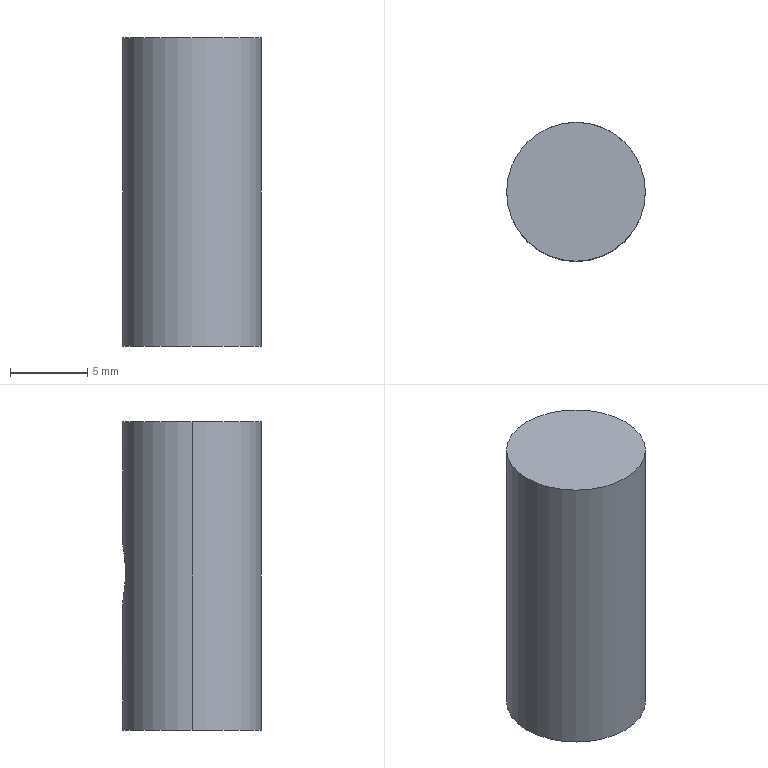Part | SolidWorks | features 3DProfileFeature 1, Extrusion 1, HoleWzd 1 | 1 solid | 8 faces | box 9 x 9 x 20 mm | volume 1148 mm3 | cylinder 4 | cone 2 | plane 2 | commonest cylinder face diameters 5 x2 9 x2
STEP:
#1=CARTESIAN_POINT('',(-0.8907,-2.867,10.19));
#2=VERTEX_POINT('',#1);
#3=CARTESIAN_POINT('',(-2.832,-0.6908,10.19));
#4=VERTEX_POINT('',#3);
#5=CARTESIAN_POINT('',(-2.832,-0.6908,10.19));
#6=DIRECTION('',(-0.6658,0.7462,0.));
#7=VECTOR('',#6,1000.);
#8=LINE('',#5,#7);
#9=EDGE_CURVE('',#2,#4,#8,.T.);
#10=ORIENTED_EDGE('',*,*,#9,.F.);
#11=CARTESIAN_POINT('',(1.942,-2.174,10.19));
#12=VERTEX_POINT('',#11);
#13=CARTESIAN_POINT('',(1.942,-2.174,10.19));
#14=DIRECTION('',(0.9714,0.2375,0.));
#15=VECTOR('',#14,1000.);
#16=LINE('',#13,#15);
#17=EDGE_CURVE('',#2,#12,#16,.T.);
#18=ORIENTED_EDGE('',*,*,#17,.T.);
#19=CARTESIAN_POINT('',(-0.445,-1.432,10.19));
#20=DIRECTION('',(0.2967,0.955,0.));
#21=DIRECTION('',(-0.955,0.2967,0.));
#22=AXIS2_PLACEMENT_3D('',#19,#20,#21);
#23=CIRCLE('',#22,2.5);
#24=EDGE_CURVE('',#12,#4,#23,.T.);
#25=ORIENTED_EDGE('',*,*,#24,.T.);
#26=EDGE_LOOP('',(#10,#18,#25));
#27=FACE_OUTER_BOUND('',#26,.T.);
#28=CARTESIAN_POINT('',(-0.445,-1.432,10.19));
#29=DIRECTION('',(0.2967,0.955,0.));
#30=DIRECTION('',(-0.955,0.2967,0.));
#31=AXIS2_PLACEMENT_3D('',#28,#29,#30);
#32=CONICAL_SURFACE('',#31,2.5,1.03);
#33=ADVANCED_FACE('',(#27),#32,.F.);
#34=ORIENTED_EDGE('',*,*,#24,.F.);
#35=CARTESIAN_POINT('',(3.498,2.831,10.19));
#36=VERTEX_POINT('',#35);
#37=CARTESIAN_POINT('',(3.723,3.556,10.19));
#38=DIRECTION('',(0.2967,0.955,0.));
#39=VECTOR('',#38,1000.);
#40=LINE('',#37,#39);
#41=EDGE_CURVE('',#12,#36,#40,.T.);
#42=ORIENTED_EDGE('',*,*,#41,.T.);
#43=CARTESIAN_POINT('',(-1.277,4.315,10.19));
#44=VERTEX_POINT('',#43);
#45=CARTESIAN_POINT('',(-1.277,4.315,10.19));
#46=CARTESIAN_POINT('',(-1.277,4.315,10.021));
#47=CARTESIAN_POINT('',(-1.258,4.321,9.855));
#48=CARTESIAN_POINT('',(-1.182,4.342,9.531));
#49=CARTESIAN_POINT('',(-1.126,4.358,9.371));
#50=CARTESIAN_POINT('',(-0.9113,4.409,8.921));
#51=CARTESIAN_POINT('',(-0.7062,4.451,8.649));
#52=CARTESIAN_POINT('',(-0.3401,4.489,8.31));
#53=CARTESIAN_POINT('',(-0.2061,4.497,8.207));
#54=CARTESIAN_POINT('',(0.07581,4.502,8.026));
#55=CARTESIAN_POINT('',(0.223,4.497,7.949));
#56=CARTESIAN_POINT('',(0.5298,4.471,7.823));
#57=CARTESIAN_POINT('',(0.6916,4.45,7.773));
#58=CARTESIAN_POINT('',(1.013,4.388,7.707));
#59=CARTESIAN_POINT('',(1.173,4.348,7.69));
#60=CARTESIAN_POINT('',(1.493,4.248,7.69));
#61=CARTESIAN_POINT('',(1.652,4.189,7.707));
#62=CARTESIAN_POINT('',(1.951,4.058,7.773));
#63=CARTESIAN_POINT('',(2.096,3.985,7.822));
#64=CARTESIAN_POINT('',(2.366,3.831,7.95));
#65=CARTESIAN_POINT('',(2.49,3.751,8.027));
#66=CARTESIAN_POINT('',(2.721,3.587,8.209));
#67=CARTESIAN_POINT('',(2.826,3.504,8.313));
#68=CARTESIAN_POINT('',(3.106,3.266,8.652));
#69=CARTESIAN_POINT('',(3.251,3.115,8.924));
#70=CARTESIAN_POINT('',(3.397,2.952,9.373));
#71=CARTESIAN_POINT('',(3.435,2.907,9.532));
#72=CARTESIAN_POINT('',(3.485,2.847,9.858));
#73=CARTESIAN_POINT('',(3.498,2.831,10.023));
#74=CARTESIAN_POINT('',(3.498,2.831,10.19));
#75=B_SPLINE_CURVE_WITH_KNOTS('',3,(#45,#46,#47,#48,#49,#50,#51,#52,#53,#54,#55,#56,#57,#58,#59,#60,#61,#62,#63,#64,#65,#66,#67,#68,#69,#70,#71,#72,#73,#74),.UNSPECIFIED.,.F.,.F.,(4,2,2,2,2,2,2,2,2,2,2,2,2,2,4),(0.,0.0004993,0.0009985,0.001997,0.002496,0.002996,0.003495,0.003994,0.004493,0.004993,0.005492,0.005991,0.00699,0.007489,0.007988),.UNSPECIFIED.);
#76=EDGE_CURVE('',#44,#36,#75,.T.);
#77=ORIENTED_EDGE('',*,*,#76,.F.);
#78=CARTESIAN_POINT('',(-1.052,5.039,10.19));
#79=DIRECTION('',(0.2967,0.955,0.));
#80=VECTOR('',#79,1000.);
#81=LINE('',#78,#80);
#82=EDGE_CURVE('',#4,#44,#81,.T.);
#83=ORIENTED_EDGE('',*,*,#82,.F.);
#84=EDGE_LOOP('',(#34,#42,#77,#83));
#85=FACE_OUTER_BOUND('',#84,.T.);
#86=CARTESIAN_POINT('',(1.335,4.297,10.19));
#87=DIRECTION('',(0.2967,0.955,0.));
#88=DIRECTION('',(-0.955,0.2967,0.));
#89=AXIS2_PLACEMENT_3D('',#86,#87,#88);
#90=CYLINDRICAL_SURFACE('',#89,2.5);
#91=ADVANCED_FACE('',(#85),#90,.F.);
#92=ORIENTED_EDGE('',*,*,#76,.T.);
#93=CARTESIAN_POINT('',(3.498,2.831,10.19));
#94=CARTESIAN_POINT('',(3.498,2.831,10.356));
#95=CARTESIAN_POINT('',(3.485,2.848,10.526));
#96=CARTESIAN_POINT('',(3.434,2.908,10.85));
#97=CARTESIAN_POINT('',(3.397,2.952,11.008));
#98=CARTESIAN_POINT('',(3.298,3.062,11.31));
#99=CARTESIAN_POINT('',(3.238,3.127,11.451));
#100=CARTESIAN_POINT('',(3.094,3.269,11.718));
#101=CARTESIAN_POINT('',(3.01,3.347,11.843));
#102=CARTESIAN_POINT('',(2.73,3.586,12.182));
#103=CARTESIAN_POINT('',(2.497,3.756,12.367));
#104=CARTESIAN_POINT('',(2.098,3.984,12.557));
#105=CARTESIAN_POINT('',(1.954,4.057,12.606));
#106=CARTESIAN_POINT('',(1.652,4.189,12.673));
#107=CARTESIAN_POINT('',(1.497,4.247,12.689));
#108=CARTESIAN_POINT('',(1.179,4.346,12.69));
#109=CARTESIAN_POINT('',(1.015,4.387,12.673));
#110=CARTESIAN_POINT('',(0.6931,4.449,12.607));
#111=CARTESIAN_POINT('',(0.5347,4.471,12.559));
#112=CARTESIAN_POINT('',(0.2234,4.497,12.43));
#113=CARTESIAN_POINT('',(0.07541,4.502,12.353));
#114=CARTESIAN_POINT('',(-0.206,4.497,12.173));
#115=CARTESIAN_POINT('',(-0.3403,4.489,12.069));
#116=CARTESIAN_POINT('',(-0.5847,4.464,11.842));
#117=CARTESIAN_POINT('',(-0.696,4.447,11.719));
#118=CARTESIAN_POINT('',(-0.8956,4.411,11.452));
#119=CARTESIAN_POINT('',(-0.9828,4.392,11.308));
#120=CARTESIAN_POINT('',(-1.125,4.358,11.01));
#121=CARTESIAN_POINT('',(-1.181,4.343,10.854));
#122=CARTESIAN_POINT('',(-1.258,4.321,10.526));
#123=CARTESIAN_POINT('',(-1.277,4.315,10.358));
#124=CARTESIAN_POINT('',(-1.277,4.315,10.19));
#125=B_SPLINE_CURVE_WITH_KNOTS('',3,(#93,#94,#95,#96,#97,#98,#99,#100,#101,#102,#103,#104,#105,#106,#107,#108,#109,#110,#111,#112,#113,#114,#115,#116,#117,#118,#119,#120,#121,#122,#123,#124),.UNSPECIFIED.,.F.,.F.,(4,2,2,2,2,2,2,2,2,2,2,2,2,2,2,4),(0.007988,0.008486,0.008984,0.009482,0.00998,0.01098,0.01147,0.01197,0.01247,0.01297,0.01347,0.01396,0.01446,0.01496,0.01546,0.01596),.UNSPECIFIED.);
#126=EDGE_CURVE('',#36,#44,#125,.T.);
#127=ORIENTED_EDGE('',*,*,#126,.T.);
#128=EDGE_LOOP('',(#92,#127));
#129=FACE_BOUND('',#128,.T.);
#130=CARTESIAN_POINT('',(4.5,0.,20.));
#131=VERTEX_POINT('',#130);
#132=CARTESIAN_POINT('',(-4.5,0.,20.));
#133=VERTEX_POINT('',#132);
#134=CARTESIAN_POINT('',(0.,0.,20.));
#135=DIRECTION('',(0.,0.,1.));
#136=DIRECTION('',(1.,0.,0.));
#137=AXIS2_PLACEMENT_3D('',#134,#135,#136);
#138=CIRCLE('',#137,4.5);
#139=EDGE_CURVE('',#131,#133,#138,.T.);
#140=ORIENTED_EDGE('',*,*,#139,.F.);
#141=CARTESIAN_POINT('',(4.5,0.,0.));
#142=VERTEX_POINT('',#141);
#143=CARTESIAN_POINT('',(4.5,0.,20.));
#144=DIRECTION('',(0.,0.,-1.));
#145=VECTOR('',#144,1000.);
#146=LINE('',#143,#145);
#147=EDGE_CURVE('',#131,#142,#146,.T.);
#148=ORIENTED_EDGE('',*,*,#147,.T.);
#149=CARTESIAN_POINT('',(-4.5,0.,0.));
#150=VERTEX_POINT('',#149);
#151=CARTESIAN_POINT('',(0.,0.,0.));
#152=DIRECTION('',(0.,0.,1.));
#153=DIRECTION('',(1.,0.,0.));
#154=AXIS2_PLACEMENT_3D('',#151,#152,#153);
#155=CIRCLE('',#154,4.5);
#156=EDGE_CURVE('',#142,#150,#155,.T.);
#157=ORIENTED_EDGE('',*,*,#156,.T.);
#158=CARTESIAN_POINT('',(-4.5,0.,20.));
#159=DIRECTION('',(0.,0.,-1.));
#160=VECTOR('',#159,1000.);
#161=LINE('',#158,#160);
#162=EDGE_CURVE('',#133,#150,#161,.T.);
#163=ORIENTED_EDGE('',*,*,#162,.F.);
#164=EDGE_LOOP('',(#140,#148,#157,#163));
#165=FACE_OUTER_BOUND('',#164,.T.);
#166=CARTESIAN_POINT('',(0.,0.,20.));
#167=DIRECTION('',(0.,0.,-1.));
#168=DIRECTION('',(-1.,0.,0.));
#169=AXIS2_PLACEMENT_3D('',#166,#167,#168);
#170=CYLINDRICAL_SURFACE('',#169,4.5);
#171=ADVANCED_FACE('',(#129,#165),#170,.T.);
#172=ORIENTED_EDGE('',*,*,#147,.F.);
#173=CARTESIAN_POINT('',(0.,0.,20.));
#174=DIRECTION('',(0.,0.,1.));
#175=DIRECTION('',(1.,0.,0.));
#176=AXIS2_PLACEMENT_3D('',#173,#174,#175);
#177=CIRCLE('',#176,4.5);
#178=EDGE_CURVE('',#133,#131,#177,.T.);
#179=ORIENTED_EDGE('',*,*,#178,.F.);
#180=ORIENTED_EDGE('',*,*,#162,.T.);
#181=CARTESIAN_POINT('',(0.,0.,0.));
#182=DIRECTION('',(0.,0.,1.));
#183=DIRECTION('',(1.,0.,0.));
#184=AXIS2_PLACEMENT_3D('',#181,#182,#183);
#185=CIRCLE('',#184,4.5);
#186=EDGE_CURVE('',#150,#142,#185,.T.);
#187=ORIENTED_EDGE('',*,*,#186,.T.);
#188=EDGE_LOOP('',(#172,#179,#180,#187));
#189=FACE_OUTER_BOUND('',#188,.T.);
#190=CARTESIAN_POINT('',(0.,0.,20.));
#191=DIRECTION('',(0.,0.,-1.));
#192=DIRECTION('',(-1.,0.,0.));
#193=AXIS2_PLACEMENT_3D('',#190,#191,#192);
#194=CYLINDRICAL_SURFACE('',#193,4.5);
#195=ADVANCED_FACE('',(#189),#194,.T.);
#196=ORIENTED_EDGE('',*,*,#178,.T.);
#197=ORIENTED_EDGE('',*,*,#139,.T.);
#198=EDGE_LOOP('',(#196,#197));
#199=FACE_OUTER_BOUND('',#198,.T.);
#200=CARTESIAN_POINT('',(0.,0.,20.));
#201=DIRECTION('',(0.,0.,1.));
#202=DIRECTION('',(1.,0.,0.));
#203=AXIS2_PLACEMENT_3D('',#200,#201,#202);
#204=PLANE('',#203);
#205=ADVANCED_FACE('',(#199),#204,.T.);
#206=ORIENTED_EDGE('',*,*,#186,.F.);
#207=ORIENTED_EDGE('',*,*,#156,.F.);
#208=EDGE_LOOP('',(#206,#207));
#209=FACE_OUTER_BOUND('',#208,.T.);
#210=CARTESIAN_POINT('',(0.,0.,0.));
#211=DIRECTION('',(0.,0.,1.));
#212=DIRECTION('',(1.,0.,0.));
#213=AXIS2_PLACEMENT_3D('',#210,#211,#212);
#214=PLANE('',#213);
#215=ADVANCED_FACE('',(#209),#214,.F.);
#216=ORIENTED_EDGE('',*,*,#41,.F.);
#217=CARTESIAN_POINT('',(-0.445,-1.432,10.19));
#218=DIRECTION('',(0.2967,0.955,0.));
#219=DIRECTION('',(-0.955,0.2967,0.));
#220=AXIS2_PLACEMENT_3D('',#217,#218,#219);
#221=CIRCLE('',#220,2.5);
#222=EDGE_CURVE('',#4,#12,#221,.T.);
#223=ORIENTED_EDGE('',*,*,#222,.F.);
#224=ORIENTED_EDGE('',*,*,#82,.T.);
#225=ORIENTED_EDGE('',*,*,#126,.F.);
#226=EDGE_LOOP('',(#216,#223,#224,#225));
#227=FACE_OUTER_BOUND('',#226,.T.);
#228=CARTESIAN_POINT('',(1.335,4.297,10.19));
#229=DIRECTION('',(0.2967,0.955,0.));
#230=DIRECTION('',(-0.955,0.2967,0.));
#231=AXIS2_PLACEMENT_3D('',#228,#229,#230);
#232=CYLINDRICAL_SURFACE('',#231,2.5);
#233=ADVANCED_FACE('',(#227),#232,.F.);
#234=ORIENTED_EDGE('',*,*,#17,.F.);
#235=ORIENTED_EDGE('',*,*,#9,.T.);
#236=ORIENTED_EDGE('',*,*,#222,.T.);
#237=EDGE_LOOP('',(#234,#235,#236));
#238=FACE_OUTER_BOUND('',#237,.T.);
#239=CARTESIAN_POINT('',(-0.445,-1.432,10.19));
#240=DIRECTION('',(0.2967,0.955,0.));
#241=DIRECTION('',(-0.955,0.2967,0.));
#242=AXIS2_PLACEMENT_3D('',#239,#240,#241);
#243=CONICAL_SURFACE('',#242,2.5,1.03);
#244=ADVANCED_FACE('',(#238),#243,.F.);
#245=CLOSED_SHELL('',(#33,#91,#171,#195,#205,#215,#233,#244));
#246=MANIFOLD_SOLID_BREP('',#245);
#247=CARTESIAN_POINT('',(0.,0.,0.));
#248=DIRECTION('',(0.,0.,1.));
#249=DIRECTION('',(1.,0.,0.));
#250=AXIS2_PLACEMENT_3D('',#247,#248,#249);
#251=(LENGTH_UNIT()NAMED_UNIT(*)SI_UNIT(.MILLI.,.METRE.));
#252=UNCERTAINTY_MEASURE_WITH_UNIT(LENGTH_MEASURE(0.00001),#251,'','');
#253=(NAMED_UNIT(*)PLANE_ANGLE_UNIT()SI_UNIT($,.RADIAN.));
#254=(NAMED_UNIT(*)SI_UNIT($,.STERADIAN.)SOLID_ANGLE_UNIT());
#255=(GEOMETRIC_REPRESENTATION_CONTEXT(3)GLOBAL_UNCERTAINTY_ASSIGNED_CONTEXT((#252))GLOBAL_UNIT_ASSIGNED_CONTEXT((#251,#253,#254))REPRESENTATION_CONTEXT('',''));
#256=ADVANCED_BREP_SHAPE_REPRESENTATION('',(#246,#250),#255);